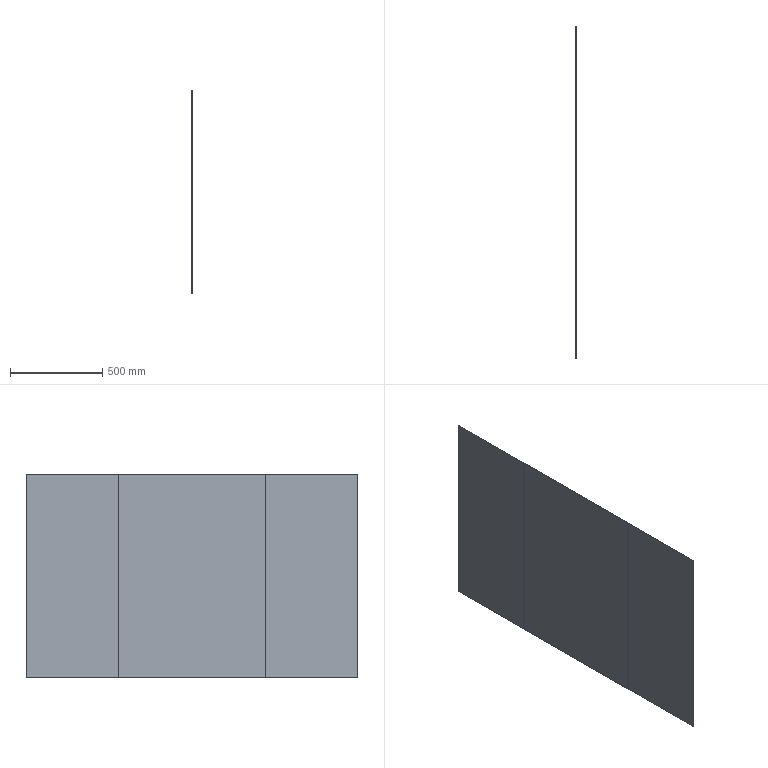Part | SolidWorks | features FlatPattern 1, SMBaseFlange 1, SheetMetal 1, UnFold 1 | 1 solid | 22 faces | box 1.2 x 1797 x 1100 mm | volume 2372141 mm3 | plane 22
STEP:
#1=CARTESIAN_POINT('',(488.189,920.05,550.));
#2=VERTEX_POINT('',#1);
#3=CARTESIAN_POINT('',(488.189,122.47,550.));
#4=VERTEX_POINT('',#3);
#5=CARTESIAN_POINT('',(488.189,921.26,550.));
#6=DIRECTION('',(0.,-1.,0.));
#7=VECTOR('',#6,1000.);
#8=LINE('',#5,#7);
#9=EDGE_CURVE('',#2,#4,#8,.T.);
#10=ORIENTED_EDGE('',*,*,#9,.F.);
#11=CARTESIAN_POINT('',(486.989,920.05,550.));
#12=VERTEX_POINT('',#11);
#13=CARTESIAN_POINT('',(488.189,920.05,550.));
#14=DIRECTION('',(-1.,0.,0.));
#15=VECTOR('',#14,1000.);
#16=LINE('',#13,#15);
#17=EDGE_CURVE('',#2,#12,#16,.T.);
#18=ORIENTED_EDGE('',*,*,#17,.T.);
#19=CARTESIAN_POINT('',(486.989,122.47,550.));
#20=VERTEX_POINT('',#19);
#21=CARTESIAN_POINT('',(486.989,921.26,550.));
#22=DIRECTION('',(0.,-1.,0.));
#23=VECTOR('',#22,1000.);
#24=LINE('',#21,#23);
#25=EDGE_CURVE('',#12,#20,#24,.T.);
#26=ORIENTED_EDGE('',*,*,#25,.T.);
#27=CARTESIAN_POINT('',(486.989,122.47,550.));
#28=DIRECTION('',(1.,0.,0.));
#29=VECTOR('',#28,1000.);
#30=LINE('',#27,#29);
#31=EDGE_CURVE('',#20,#4,#30,.T.);
#32=ORIENTED_EDGE('',*,*,#31,.T.);
#33=EDGE_LOOP('',(#10,#18,#26,#32));
#34=FACE_OUTER_BOUND('',#33,.T.);
#35=CARTESIAN_POINT('',(486.979,920.06,550.));
#36=DIRECTION('',(0.,0.,1.));
#37=DIRECTION('',(1.,0.,0.));
#38=AXIS2_PLACEMENT_3D('',#35,#36,#37);
#39=PLANE('',#38);
#40=ADVANCED_FACE('',(#34),#39,.T.);
#41=CARTESIAN_POINT('',(488.189,920.05,-550.));
#42=VERTEX_POINT('',#41);
#43=CARTESIAN_POINT('',(488.189,122.47,-550.));
#44=VERTEX_POINT('',#43);
#45=CARTESIAN_POINT('',(488.189,921.26,-550.));
#46=DIRECTION('',(0.,-1.,0.));
#47=VECTOR('',#46,1000.);
#48=LINE('',#45,#47);
#49=EDGE_CURVE('',#42,#44,#48,.T.);
#50=ORIENTED_EDGE('',*,*,#49,.T.);
#51=CARTESIAN_POINT('',(486.989,122.47,-550.));
#52=VERTEX_POINT('',#51);
#53=CARTESIAN_POINT('',(488.189,122.47,-550.));
#54=DIRECTION('',(-1.,0.,0.));
#55=VECTOR('',#54,1000.);
#56=LINE('',#53,#55);
#57=EDGE_CURVE('',#44,#52,#56,.T.);
#58=ORIENTED_EDGE('',*,*,#57,.T.);
#59=CARTESIAN_POINT('',(486.989,920.05,-550.));
#60=VERTEX_POINT('',#59);
#61=CARTESIAN_POINT('',(486.989,921.26,-550.));
#62=DIRECTION('',(0.,-1.,0.));
#63=VECTOR('',#62,1000.);
#64=LINE('',#61,#63);
#65=EDGE_CURVE('',#60,#52,#64,.T.);
#66=ORIENTED_EDGE('',*,*,#65,.F.);
#67=CARTESIAN_POINT('',(486.989,920.05,-550.));
#68=DIRECTION('',(1.,0.,0.));
#69=VECTOR('',#68,1000.);
#70=LINE('',#67,#69);
#71=EDGE_CURVE('',#60,#42,#70,.T.);
#72=ORIENTED_EDGE('',*,*,#71,.T.);
#73=EDGE_LOOP('',(#50,#58,#66,#72));
#74=FACE_OUTER_BOUND('',#73,.T.);
#75=CARTESIAN_POINT('',(486.979,122.46,-550.));
#76=DIRECTION('',(0.,0.,-1.));
#77=DIRECTION('',(-1.,0.,0.));
#78=AXIS2_PLACEMENT_3D('',#75,#76,#77);
#79=PLANE('',#78);
#80=ADVANCED_FACE('',(#74),#79,.T.);
#81=ORIENTED_EDGE('',*,*,#49,.F.);
#82=CARTESIAN_POINT('',(488.189,920.05,550.));
#83=DIRECTION('',(0.,0.,-1.));
#84=VECTOR('',#83,1000.);
#85=LINE('',#82,#84);
#86=EDGE_CURVE('',#2,#42,#85,.T.);
#87=ORIENTED_EDGE('',*,*,#86,.F.);
#88=ORIENTED_EDGE('',*,*,#9,.T.);
#89=CARTESIAN_POINT('',(488.189,122.47,550.));
#90=DIRECTION('',(0.,0.,-1.));
#91=VECTOR('',#90,1000.);
#92=LINE('',#89,#91);
#93=EDGE_CURVE('',#4,#44,#92,.T.);
#94=ORIENTED_EDGE('',*,*,#93,.T.);
#95=EDGE_LOOP('',(#81,#87,#88,#94));
#96=FACE_OUTER_BOUND('',#95,.T.);
#97=CARTESIAN_POINT('',(488.189,921.26,550.));
#98=DIRECTION('',(1.,0.,0.));
#99=DIRECTION('',(0.,0.,-1.));
#100=AXIS2_PLACEMENT_3D('',#97,#98,#99);
#101=PLANE('',#100);
#102=ADVANCED_FACE('',(#96),#101,.T.);
#103=ORIENTED_EDGE('',*,*,#65,.T.);
#104=CARTESIAN_POINT('',(486.989,122.47,550.));
#105=DIRECTION('',(0.,0.,-1.));
#106=VECTOR('',#105,1000.);
#107=LINE('',#104,#106);
#108=EDGE_CURVE('',#20,#52,#107,.T.);
#109=ORIENTED_EDGE('',*,*,#108,.F.);
#110=ORIENTED_EDGE('',*,*,#25,.F.);
#111=CARTESIAN_POINT('',(486.989,920.05,550.));
#112=DIRECTION('',(0.,0.,-1.));
#113=VECTOR('',#112,1000.);
#114=LINE('',#111,#113);
#115=EDGE_CURVE('',#12,#60,#114,.T.);
#116=ORIENTED_EDGE('',*,*,#115,.T.);
#117=EDGE_LOOP('',(#103,#109,#110,#116));
#118=FACE_OUTER_BOUND('',#117,.T.);
#119=CARTESIAN_POINT('',(486.989,921.26,550.));
#120=DIRECTION('',(1.,0.,0.));
#121=DIRECTION('',(0.,0.,-1.));
#122=AXIS2_PLACEMENT_3D('',#119,#120,#121);
#123=PLANE('',#122);
#124=ADVANCED_FACE('',(#118),#123,.F.);
#125=ORIENTED_EDGE('',*,*,#71,.F.);
#126=CARTESIAN_POINT('',(486.989,921.008,-550.));
#127=VERTEX_POINT('',#126);
#128=CARTESIAN_POINT('',(486.989,920.529,-550.));
#129=DIRECTION('',(0.,1.,0.));
#130=VECTOR('',#129,1000.);
#131=LINE('',#128,#130);
#132=EDGE_CURVE('',#60,#127,#131,.T.);
#133=ORIENTED_EDGE('',*,*,#132,.T.);
#134=CARTESIAN_POINT('',(488.189,921.008,-550.));
#135=VERTEX_POINT('',#134);
#136=CARTESIAN_POINT('',(488.189,921.008,-550.));
#137=DIRECTION('',(-1.,0.,0.));
#138=VECTOR('',#137,1000.);
#139=LINE('',#136,#138);
#140=EDGE_CURVE('',#135,#127,#139,.T.);
#141=ORIENTED_EDGE('',*,*,#140,.F.);
#142=CARTESIAN_POINT('',(488.189,921.008,-550.));
#143=DIRECTION('',(0.,1.,0.));
#144=VECTOR('',#143,1000.);
#145=LINE('',#142,#144);
#146=EDGE_CURVE('',#42,#135,#145,.T.);
#147=ORIENTED_EDGE('',*,*,#146,.F.);
#148=EDGE_LOOP('',(#125,#133,#141,#147));
#149=FACE_OUTER_BOUND('',#148,.T.);
#150=CARTESIAN_POINT('',(488.189,921.008,-550.));
#151=DIRECTION('',(0.,0.,-1.));
#152=DIRECTION('',(0.,1.,0.));
#153=AXIS2_PLACEMENT_3D('',#150,#151,#152);
#154=PLANE('',#153);
#155=ADVANCED_FACE('',(#149),#154,.T.);
#156=CARTESIAN_POINT('',(486.989,921.008,550.));
#157=VERTEX_POINT('',#156);
#158=CARTESIAN_POINT('',(488.189,921.008,550.));
#159=VERTEX_POINT('',#158);
#160=CARTESIAN_POINT('',(486.989,921.008,550.));
#161=DIRECTION('',(1.,0.,0.));
#162=VECTOR('',#161,1000.);
#163=LINE('',#160,#162);
#164=EDGE_CURVE('',#157,#159,#163,.T.);
#165=ORIENTED_EDGE('',*,*,#164,.F.);
#166=CARTESIAN_POINT('',(486.989,920.529,550.));
#167=DIRECTION('',(0.,-1.,0.));
#168=VECTOR('',#167,1000.);
#169=LINE('',#166,#168);
#170=EDGE_CURVE('',#157,#12,#169,.T.);
#171=ORIENTED_EDGE('',*,*,#170,.T.);
#172=ORIENTED_EDGE('',*,*,#17,.F.);
#173=CARTESIAN_POINT('',(488.189,921.008,550.));
#174=DIRECTION('',(0.,-1.,0.));
#175=VECTOR('',#174,1000.);
#176=LINE('',#173,#175);
#177=EDGE_CURVE('',#159,#2,#176,.T.);
#178=ORIENTED_EDGE('',*,*,#177,.F.);
#179=EDGE_LOOP('',(#165,#171,#172,#178));
#180=FACE_OUTER_BOUND('',#179,.T.);
#181=CARTESIAN_POINT('',(488.189,921.008,550.));
#182=DIRECTION('',(0.,0.,1.));
#183=DIRECTION('',(0.,-1.,0.));
#184=AXIS2_PLACEMENT_3D('',#181,#182,#183);
#185=PLANE('',#184);
#186=ADVANCED_FACE('',(#180),#185,.T.);
#187=ORIENTED_EDGE('',*,*,#177,.T.);
#188=ORIENTED_EDGE('',*,*,#86,.T.);
#189=ORIENTED_EDGE('',*,*,#146,.T.);
#190=CARTESIAN_POINT('',(488.189,921.008,550.));
#191=DIRECTION('',(0.,0.,-1.));
#192=VECTOR('',#191,1000.);
#193=LINE('',#190,#192);
#194=EDGE_CURVE('',#159,#135,#193,.T.);
#195=ORIENTED_EDGE('',*,*,#194,.F.);
#196=EDGE_LOOP('',(#187,#188,#189,#195));
#197=FACE_OUTER_BOUND('',#196,.T.);
#198=CARTESIAN_POINT('',(488.189,920.529,0.));
#199=DIRECTION('',(1.,0.,0.));
#200=DIRECTION('',(0.,0.,-1.));
#201=AXIS2_PLACEMENT_3D('',#198,#199,#200);
#202=PLANE('',#201);
#203=ADVANCED_FACE('',(#197),#202,.T.);
#204=ORIENTED_EDGE('',*,*,#170,.F.);
#205=CARTESIAN_POINT('',(486.989,921.008,550.));
#206=DIRECTION('',(0.,0.,-1.));
#207=VECTOR('',#206,1000.);
#208=LINE('',#205,#207);
#209=EDGE_CURVE('',#157,#127,#208,.T.);
#210=ORIENTED_EDGE('',*,*,#209,.T.);
#211=ORIENTED_EDGE('',*,*,#132,.F.);
#212=ORIENTED_EDGE('',*,*,#115,.F.);
#213=EDGE_LOOP('',(#204,#210,#211,#212));
#214=FACE_OUTER_BOUND('',#213,.T.);
#215=CARTESIAN_POINT('',(486.989,920.529,0.));
#216=DIRECTION('',(1.,0.,0.));
#217=DIRECTION('',(0.,0.,-1.));
#218=AXIS2_PLACEMENT_3D('',#215,#216,#217);
#219=PLANE('',#218);
#220=ADVANCED_FACE('',(#214),#219,.F.);
#221=CARTESIAN_POINT('',(486.989,1419.798,-550.));
#222=VERTEX_POINT('',#221);
#223=CARTESIAN_POINT('',(488.189,1419.798,-550.));
#224=VERTEX_POINT('',#223);
#225=CARTESIAN_POINT('',(486.989,1419.798,-550.));
#226=DIRECTION('',(1.,0.,0.));
#227=VECTOR('',#226,1000.);
#228=LINE('',#225,#227);
#229=EDGE_CURVE('',#222,#224,#228,.T.);
#230=ORIENTED_EDGE('',*,*,#229,.F.);
#231=CARTESIAN_POINT('',(486.989,1419.798,550.));
#232=VERTEX_POINT('',#231);
#233=CARTESIAN_POINT('',(486.989,1419.798,550.));
#234=DIRECTION('',(0.,0.,-1.));
#235=VECTOR('',#234,1000.);
#236=LINE('',#233,#235);
#237=EDGE_CURVE('',#232,#222,#236,.T.);
#238=ORIENTED_EDGE('',*,*,#237,.F.);
#239=CARTESIAN_POINT('',(488.189,1419.798,550.));
#240=VERTEX_POINT('',#239);
#241=CARTESIAN_POINT('',(486.989,1419.798,550.));
#242=DIRECTION('',(1.,0.,0.));
#243=VECTOR('',#242,1000.);
#244=LINE('',#241,#243);
#245=EDGE_CURVE('',#232,#240,#244,.T.);
#246=ORIENTED_EDGE('',*,*,#245,.T.);
#247=CARTESIAN_POINT('',(488.189,1419.798,550.));
#248=DIRECTION('',(0.,0.,-1.));
#249=VECTOR('',#248,1000.);
#250=LINE('',#247,#249);
#251=EDGE_CURVE('',#240,#224,#250,.T.);
#252=ORIENTED_EDGE('',*,*,#251,.T.);
#253=EDGE_LOOP('',(#230,#238,#246,#252));
#254=FACE_OUTER_BOUND('',#253,.T.);
#255=CARTESIAN_POINT('',(486.989,1419.798,550.));
#256=DIRECTION('',(0.,1.,0.));
#257=DIRECTION('',(0.,0.,1.));
#258=AXIS2_PLACEMENT_3D('',#255,#256,#257);
#259=PLANE('',#258);
#260=ADVANCED_FACE('',(#254),#259,.T.);
#261=CARTESIAN_POINT('',(488.189,1419.798,-550.));
#262=DIRECTION('',(0.,-1.,0.));
#263=VECTOR('',#262,1000.);
#264=LINE('',#261,#263);
#265=EDGE_CURVE('',#224,#135,#264,.T.);
#266=ORIENTED_EDGE('',*,*,#265,.F.);
#267=ORIENTED_EDGE('',*,*,#251,.F.);
#268=CARTESIAN_POINT('',(488.189,1419.798,550.));
#269=DIRECTION('',(0.,-1.,0.));
#270=VECTOR('',#269,1000.);
#271=LINE('',#268,#270);
#272=EDGE_CURVE('',#240,#159,#271,.T.);
#273=ORIENTED_EDGE('',*,*,#272,.T.);
#274=ORIENTED_EDGE('',*,*,#194,.T.);
#275=EDGE_LOOP('',(#266,#267,#273,#274));
#276=FACE_OUTER_BOUND('',#275,.T.);
#277=CARTESIAN_POINT('',(488.189,1419.798,550.));
#278=DIRECTION('',(1.,0.,0.));
#279=DIRECTION('',(0.,0.,1.));
#280=AXIS2_PLACEMENT_3D('',#277,#278,#279);
#281=PLANE('',#280);
#282=ADVANCED_FACE('',(#276),#281,.T.);
#283=ORIENTED_EDGE('',*,*,#265,.T.);
#284=ORIENTED_EDGE('',*,*,#140,.T.);
#285=CARTESIAN_POINT('',(486.989,1419.798,-550.));
#286=DIRECTION('',(0.,-1.,0.));
#287=VECTOR('',#286,1000.);
#288=LINE('',#285,#287);
#289=EDGE_CURVE('',#222,#127,#288,.T.);
#290=ORIENTED_EDGE('',*,*,#289,.F.);
#291=ORIENTED_EDGE('',*,*,#229,.T.);
#292=EDGE_LOOP('',(#283,#284,#290,#291));
#293=FACE_OUTER_BOUND('',#292,.T.);
#294=CARTESIAN_POINT('',(486.979,920.998,-550.));
#295=DIRECTION('',(0.,0.,-1.));
#296=DIRECTION('',(0.,1.,0.));
#297=AXIS2_PLACEMENT_3D('',#294,#295,#296);
#298=PLANE('',#297);
#299=ADVANCED_FACE('',(#293),#298,.T.);
#300=ORIENTED_EDGE('',*,*,#289,.T.);
#301=ORIENTED_EDGE('',*,*,#209,.F.);
#302=CARTESIAN_POINT('',(486.989,1419.798,550.));
#303=DIRECTION('',(0.,-1.,0.));
#304=VECTOR('',#303,1000.);
#305=LINE('',#302,#304);
#306=EDGE_CURVE('',#232,#157,#305,.T.);
#307=ORIENTED_EDGE('',*,*,#306,.F.);
#308=ORIENTED_EDGE('',*,*,#237,.T.);
#309=EDGE_LOOP('',(#300,#301,#307,#308));
#310=FACE_OUTER_BOUND('',#309,.T.);
#311=CARTESIAN_POINT('',(486.989,1419.798,550.));
#312=DIRECTION('',(1.,0.,0.));
#313=DIRECTION('',(0.,0.,1.));
#314=AXIS2_PLACEMENT_3D('',#311,#312,#313);
#315=PLANE('',#314);
#316=ADVANCED_FACE('',(#310),#315,.F.);
#317=ORIENTED_EDGE('',*,*,#306,.T.);
#318=ORIENTED_EDGE('',*,*,#164,.T.);
#319=ORIENTED_EDGE('',*,*,#272,.F.);
#320=ORIENTED_EDGE('',*,*,#245,.F.);
#321=EDGE_LOOP('',(#317,#318,#319,#320));
#322=FACE_OUTER_BOUND('',#321,.T.);
#323=CARTESIAN_POINT('',(-310.601,921.008,550.));
#324=DIRECTION('',(0.,0.,1.));
#325=DIRECTION('',(0.,-1.,0.));
#326=AXIS2_PLACEMENT_3D('',#323,#324,#325);
#327=PLANE('',#326);
#328=ADVANCED_FACE('',(#322),#327,.T.);
#329=CARTESIAN_POINT('',(486.989,121.512,-550.));
#330=VERTEX_POINT('',#329);
#331=CARTESIAN_POINT('',(488.189,121.512,-550.));
#332=VERTEX_POINT('',#331);
#333=CARTESIAN_POINT('',(486.989,121.512,-550.));
#334=DIRECTION('',(1.,0.,0.));
#335=VECTOR('',#334,1000.);
#336=LINE('',#333,#335);
#337=EDGE_CURVE('',#330,#332,#336,.T.);
#338=ORIENTED_EDGE('',*,*,#337,.F.);
#339=CARTESIAN_POINT('',(486.989,121.991,-550.));
#340=DIRECTION('',(0.,1.,0.));
#341=VECTOR('',#340,1000.);
#342=LINE('',#339,#341);
#343=EDGE_CURVE('',#330,#52,#342,.T.);
#344=ORIENTED_EDGE('',*,*,#343,.T.);
#345=ORIENTED_EDGE('',*,*,#57,.F.);
#346=CARTESIAN_POINT('',(488.189,122.47,-550.));
#347=DIRECTION('',(0.,1.,0.));
#348=VECTOR('',#347,1000.);
#349=LINE('',#346,#348);
#350=EDGE_CURVE('',#332,#44,#349,.T.);
#351=ORIENTED_EDGE('',*,*,#350,.F.);
#352=EDGE_LOOP('',(#338,#344,#345,#351));
#353=FACE_OUTER_BOUND('',#352,.T.);
#354=CARTESIAN_POINT('',(488.189,122.47,-550.));
#355=DIRECTION('',(0.,0.,-1.));
#356=DIRECTION('',(0.,1.,0.));
#357=AXIS2_PLACEMENT_3D('',#354,#355,#356);
#358=PLANE('',#357);
#359=ADVANCED_FACE('',(#353),#358,.T.);
#360=ORIENTED_EDGE('',*,*,#31,.F.);
#361=CARTESIAN_POINT('',(486.989,121.512,550.));
#362=VERTEX_POINT('',#361);
#363=CARTESIAN_POINT('',(486.989,121.991,550.));
#364=DIRECTION('',(0.,-1.,0.));
#365=VECTOR('',#364,1000.);
#366=LINE('',#363,#365);
#367=EDGE_CURVE('',#20,#362,#366,.T.);
#368=ORIENTED_EDGE('',*,*,#367,.T.);
#369=CARTESIAN_POINT('',(488.189,121.512,550.));
#370=VERTEX_POINT('',#369);
#371=CARTESIAN_POINT('',(488.189,121.512,550.));
#372=DIRECTION('',(-1.,0.,0.));
#373=VECTOR('',#372,1000.);
#374=LINE('',#371,#373);
#375=EDGE_CURVE('',#370,#362,#374,.T.);
#376=ORIENTED_EDGE('',*,*,#375,.F.);
#377=CARTESIAN_POINT('',(488.189,122.47,550.));
#378=DIRECTION('',(0.,-1.,0.));
#379=VECTOR('',#378,1000.);
#380=LINE('',#377,#379);
#381=EDGE_CURVE('',#4,#370,#380,.T.);
#382=ORIENTED_EDGE('',*,*,#381,.F.);
#383=EDGE_LOOP('',(#360,#368,#376,#382));
#384=FACE_OUTER_BOUND('',#383,.T.);
#385=CARTESIAN_POINT('',(488.189,122.47,550.));
#386=DIRECTION('',(0.,0.,1.));
#387=DIRECTION('',(0.,-1.,0.));
#388=AXIS2_PLACEMENT_3D('',#385,#386,#387);
#389=PLANE('',#388);
#390=ADVANCED_FACE('',(#384),#389,.T.);
#391=ORIENTED_EDGE('',*,*,#381,.T.);
#392=CARTESIAN_POINT('',(488.189,121.512,550.));
#393=DIRECTION('',(0.,0.,-1.));
#394=VECTOR('',#393,1000.);
#395=LINE('',#392,#394);
#396=EDGE_CURVE('',#370,#332,#395,.T.);
#397=ORIENTED_EDGE('',*,*,#396,.T.);
#398=ORIENTED_EDGE('',*,*,#350,.T.);
#399=ORIENTED_EDGE('',*,*,#93,.F.);
#400=EDGE_LOOP('',(#391,#397,#398,#399));
#401=FACE_OUTER_BOUND('',#400,.T.);
#402=CARTESIAN_POINT('',(488.189,121.991,0.));
#403=DIRECTION('',(1.,0.,0.));
#404=DIRECTION('',(0.,0.,-1.));
#405=AXIS2_PLACEMENT_3D('',#402,#403,#404);
#406=PLANE('',#405);
#407=ADVANCED_FACE('',(#401),#406,.T.);
#408=ORIENTED_EDGE('',*,*,#367,.F.);
#409=ORIENTED_EDGE('',*,*,#108,.T.);
#410=ORIENTED_EDGE('',*,*,#343,.F.);
#411=CARTESIAN_POINT('',(486.989,121.512,550.));
#412=DIRECTION('',(0.,0.,-1.));
#413=VECTOR('',#412,1000.);
#414=LINE('',#411,#413);
#415=EDGE_CURVE('',#362,#330,#414,.T.);
#416=ORIENTED_EDGE('',*,*,#415,.F.);
#417=EDGE_LOOP('',(#408,#409,#410,#416));
#418=FACE_OUTER_BOUND('',#417,.T.);
#419=CARTESIAN_POINT('',(486.989,121.991,0.));
#420=DIRECTION('',(1.,0.,0.));
#421=DIRECTION('',(0.,0.,-1.));
#422=AXIS2_PLACEMENT_3D('',#419,#420,#421);
#423=PLANE('',#422);
#424=ADVANCED_FACE('',(#418),#423,.F.);
#425=CARTESIAN_POINT('',(488.189,-377.278,-550.));
#426=VERTEX_POINT('',#425);
#427=CARTESIAN_POINT('',(486.989,-377.278,-550.));
#428=VERTEX_POINT('',#427);
#429=CARTESIAN_POINT('',(488.189,-377.278,-550.));
#430=DIRECTION('',(-1.,0.,0.));
#431=VECTOR('',#430,1000.);
#432=LINE('',#429,#431);
#433=EDGE_CURVE('',#426,#428,#432,.T.);
#434=ORIENTED_EDGE('',*,*,#433,.F.);
#435=CARTESIAN_POINT('',(488.189,-377.278,550.));
#436=VERTEX_POINT('',#435);
#437=CARTESIAN_POINT('',(488.189,-377.278,550.));
#438=DIRECTION('',(0.,0.,-1.));
#439=VECTOR('',#438,1000.);
#440=LINE('',#437,#439);
#441=EDGE_CURVE('',#436,#426,#440,.T.);
#442=ORIENTED_EDGE('',*,*,#441,.F.);
#443=CARTESIAN_POINT('',(486.989,-377.278,550.));
#444=VERTEX_POINT('',#443);
#445=CARTESIAN_POINT('',(488.189,-377.278,550.));
#446=DIRECTION('',(-1.,0.,0.));
#447=VECTOR('',#446,1000.);
#448=LINE('',#445,#447);
#449=EDGE_CURVE('',#436,#444,#448,.T.);
#450=ORIENTED_EDGE('',*,*,#449,.T.);
#451=CARTESIAN_POINT('',(486.989,-377.278,550.));
#452=DIRECTION('',(0.,0.,-1.));
#453=VECTOR('',#452,1000.);
#454=LINE('',#451,#453);
#455=EDGE_CURVE('',#444,#428,#454,.T.);
#456=ORIENTED_EDGE('',*,*,#455,.T.);
#457=EDGE_LOOP('',(#434,#442,#450,#456));
#458=FACE_OUTER_BOUND('',#457,.T.);
#459=CARTESIAN_POINT('',(488.189,-377.278,550.));
#460=DIRECTION('',(0.,-1.,0.));
#461=DIRECTION('',(0.,0.,1.));
#462=AXIS2_PLACEMENT_3D('',#459,#460,#461);
#463=PLANE('',#462);
#464=ADVANCED_FACE('',(#458),#463,.T.);
#465=CARTESIAN_POINT('',(488.189,122.722,-550.));
#466=DIRECTION('',(0.,-1.,0.));
#467=VECTOR('',#466,1000.);
#468=LINE('',#465,#467);
#469=EDGE_CURVE('',#332,#426,#468,.T.);
#470=ORIENTED_EDGE('',*,*,#469,.F.);
#471=ORIENTED_EDGE('',*,*,#396,.F.);
#472=CARTESIAN_POINT('',(488.189,122.722,550.));
#473=DIRECTION('',(0.,-1.,0.));
#474=VECTOR('',#473,1000.);
#475=LINE('',#472,#474);
#476=EDGE_CURVE('',#370,#436,#475,.T.);
#477=ORIENTED_EDGE('',*,*,#476,.T.);
#478=ORIENTED_EDGE('',*,*,#441,.T.);
#479=EDGE_LOOP('',(#470,#471,#477,#478));
#480=FACE_OUTER_BOUND('',#479,.T.);
#481=CARTESIAN_POINT('',(488.189,122.722,550.));
#482=DIRECTION('',(1.,0.,0.));
#483=DIRECTION('',(0.,1.,0.));
#484=AXIS2_PLACEMENT_3D('',#481,#482,#483);
#485=PLANE('',#484);
#486=ADVANCED_FACE('',(#480),#485,.T.);
#487=ORIENTED_EDGE('',*,*,#476,.F.);
#488=ORIENTED_EDGE('',*,*,#375,.T.);
#489=CARTESIAN_POINT('',(486.989,122.722,550.));
#490=DIRECTION('',(0.,-1.,0.));
#491=VECTOR('',#490,1000.);
#492=LINE('',#489,#491);
#493=EDGE_CURVE('',#362,#444,#492,.T.);
#494=ORIENTED_EDGE('',*,*,#493,.T.);
#495=ORIENTED_EDGE('',*,*,#449,.F.);
#496=EDGE_LOOP('',(#487,#488,#494,#495));
#497=FACE_OUTER_BOUND('',#496,.T.);
#498=CARTESIAN_POINT('',(486.979,121.522,550.));
#499=DIRECTION('',(0.,0.,1.));
#500=DIRECTION('',(0.,1.,0.));
#501=AXIS2_PLACEMENT_3D('',#498,#499,#500);
#502=PLANE('',#501);
#503=ADVANCED_FACE('',(#497),#502,.T.);
#504=CARTESIAN_POINT('',(486.989,122.722,-550.));
#505=DIRECTION('',(0.,-1.,0.));
#506=VECTOR('',#505,1000.);
#507=LINE('',#504,#506);
#508=EDGE_CURVE('',#330,#428,#507,.T.);
#509=ORIENTED_EDGE('',*,*,#508,.T.);
#510=ORIENTED_EDGE('',*,*,#455,.F.);
#511=ORIENTED_EDGE('',*,*,#493,.F.);
#512=ORIENTED_EDGE('',*,*,#415,.T.);
#513=EDGE_LOOP('',(#509,#510,#511,#512));
#514=FACE_OUTER_BOUND('',#513,.T.);
#515=CARTESIAN_POINT('',(486.989,122.722,550.));
#516=DIRECTION('',(1.,0.,0.));
#517=DIRECTION('',(0.,1.,0.));
#518=AXIS2_PLACEMENT_3D('',#515,#516,#517);
#519=PLANE('',#518);
#520=ADVANCED_FACE('',(#514),#519,.F.);
#521=ORIENTED_EDGE('',*,*,#508,.F.);
#522=ORIENTED_EDGE('',*,*,#337,.T.);
#523=ORIENTED_EDGE('',*,*,#469,.T.);
#524=ORIENTED_EDGE('',*,*,#433,.T.);
#525=EDGE_LOOP('',(#521,#522,#523,#524));
#526=FACE_OUTER_BOUND('',#525,.T.);
#527=CARTESIAN_POINT('',(486.979,121.512,-550.));
#528=DIRECTION('',(0.,0.,1.));
#529=DIRECTION('',(0.,1.,0.));
#530=AXIS2_PLACEMENT_3D('',#527,#528,#529);
#531=PLANE('',#530);
#532=ADVANCED_FACE('',(#526),#531,.F.);
#533=CLOSED_SHELL('',(#40,#80,#102,#124,#155,#186,#203,#220,#260,#282,#299,#316,#328,#359,#390,#407,#424,#464,#486,#503,#520,#532));
#534=MANIFOLD_SOLID_BREP('',#533);
#535=CARTESIAN_POINT('',(0.,0.,0.));
#536=DIRECTION('',(0.,0.,1.));
#537=DIRECTION('',(1.,0.,0.));
#538=AXIS2_PLACEMENT_3D('',#535,#536,#537);
#539=(LENGTH_UNIT()NAMED_UNIT(*)SI_UNIT(.MILLI.,.METRE.));
#540=UNCERTAINTY_MEASURE_WITH_UNIT(LENGTH_MEASURE(0.00001),#539,'','');
#541=(NAMED_UNIT(*)PLANE_ANGLE_UNIT()SI_UNIT($,.RADIAN.));
#542=(NAMED_UNIT(*)SI_UNIT($,.STERADIAN.)SOLID_ANGLE_UNIT());
#543=(GEOMETRIC_REPRESENTATION_CONTEXT(3)GLOBAL_UNCERTAINTY_ASSIGNED_CONTEXT((#540))GLOBAL_UNIT_ASSIGNED_CONTEXT((#539,#541,#542))REPRESENTATION_CONTEXT('',''));
#544=ADVANCED_BREP_SHAPE_REPRESENTATION('',(#534,#538),#543);